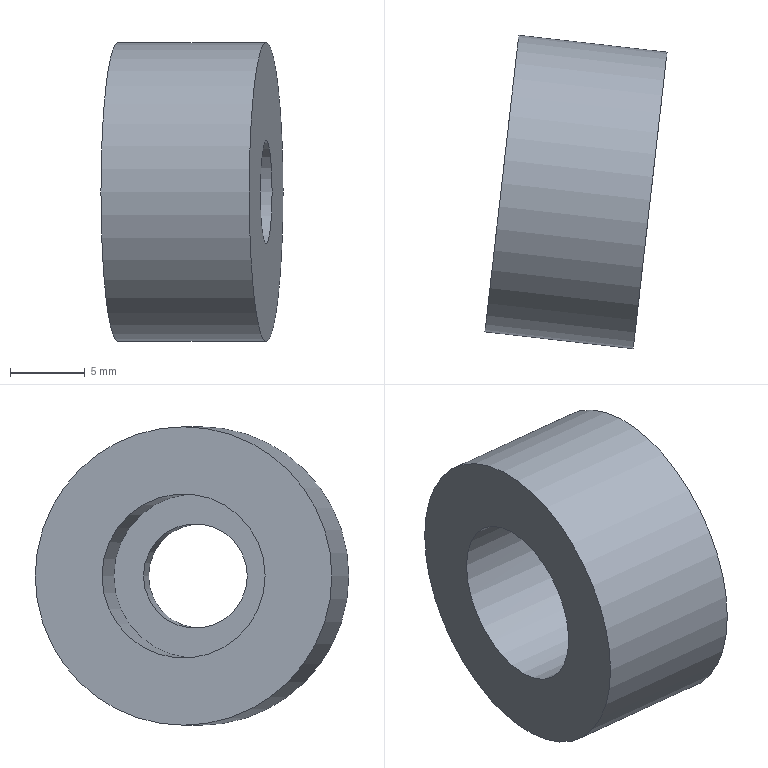Part | NX | features XQ 2 | 1 solid | 6 faces | box 12.2 x 21.003 x 20 mm | volume 2361 mm3 | plane 3 | cylinder 3 | commonest cylinder face diameters 7 x1 11 x1 20 x1
STEP:
#1=CARTESIAN_POINT('',(3212.648,-240.802,-118.5));
#2=VERTEX_POINT('',#1);
#3=CARTESIAN_POINT('',(3213.78,-230.866,-118.5));
#4=DIRECTION('',(-0.9936,0.1132,0.));
#5=DIRECTION('',(-0.1132,-0.9936,0.));
#6=AXIS2_PLACEMENT_3D('',#3,#4,#5);
#7=CIRCLE('',#6,10.);
#8=EDGE_CURVE('',#2,#2,#7,.T.);
#9=ORIENTED_EDGE('',*,*,#8,.T.);
#10=EDGE_LOOP('',(#9));
#11=FACE_BOUND('',#10,.T.);
#12=CARTESIAN_POINT('',(3213.85,-230.247,-123.965));
#13=VERTEX_POINT('',#12);
#14=CARTESIAN_POINT('',(3213.78,-230.866,-118.5));
#15=DIRECTION('',(0.9936,-0.1132,0.));
#16=DIRECTION('',(0.01281,0.1125,-0.9936));
#17=AXIS2_PLACEMENT_3D('',#14,#15,#16);
#18=CIRCLE('',#17,5.5);
#19=EDGE_CURVE('',#13,#13,#18,.T.);
#20=ORIENTED_EDGE('',*,*,#19,.T.);
#21=EDGE_LOOP('',(#20));
#22=FACE_BOUND('',#21,.T.);
#23=CARTESIAN_POINT('',(3213.78,-230.866,-118.5));
#24=DIRECTION('',(-0.9936,0.1132,0.));
#25=DIRECTION('',(0.1132,0.9936,0.));
#26=AXIS2_PLACEMENT_3D('',#23,#24,#25);
#27=PLANE('',#26);
#28=ADVANCED_FACE('',(#11,#22),#27,.T.);
#29=ORIENTED_EDGE('',*,*,#8,.F.);
#30=EDGE_LOOP('',(#29));
#31=FACE_BOUND('',#30,.T.);
#32=CARTESIAN_POINT('',(3222.584,-241.934,-118.5));
#33=VERTEX_POINT('',#32);
#34=CARTESIAN_POINT('',(3223.716,-231.998,-118.5));
#35=DIRECTION('',(-0.9936,0.1132,0.));
#36=DIRECTION('',(-0.1132,-0.9936,0.));
#37=AXIS2_PLACEMENT_3D('',#34,#35,#36);
#38=CIRCLE('',#37,10.);
#39=EDGE_CURVE('',#33,#33,#38,.T.);
#40=ORIENTED_EDGE('',*,*,#39,.T.);
#41=EDGE_LOOP('',(#40));
#42=FACE_BOUND('',#41,.T.);
#43=CARTESIAN_POINT('',(3213.78,-230.866,-118.5));
#44=DIRECTION('',(0.9936,-0.1132,0.));
#45=DIRECTION('',(-0.1132,-0.9936,0.));
#46=AXIS2_PLACEMENT_3D('',#43,#44,#45);
#47=CYLINDRICAL_SURFACE('',#46,10.);
#48=ADVANCED_FACE('',(#31,#42),#47,.T.);
#49=CARTESIAN_POINT('',(3223.319,-235.475,-118.5));
#50=VERTEX_POINT('',#49);
#51=CARTESIAN_POINT('',(3223.716,-231.998,-118.5));
#52=DIRECTION('',(-0.9936,0.1132,0.));
#53=DIRECTION('',(-0.1132,-0.9936,0.));
#54=AXIS2_PLACEMENT_3D('',#51,#52,#53);
#55=CIRCLE('',#54,3.5);
#56=EDGE_CURVE('',#50,#50,#55,.T.);
#57=ORIENTED_EDGE('',*,*,#56,.T.);
#58=EDGE_LOOP('',(#57));
#59=FACE_BOUND('',#58,.T.);
#60=ORIENTED_EDGE('',*,*,#39,.F.);
#61=EDGE_LOOP('',(#60));
#62=FACE_BOUND('',#61,.T.);
#63=CARTESIAN_POINT('',(3223.716,-231.998,-118.5));
#64=DIRECTION('',(-0.9936,0.1132,0.));
#65=DIRECTION('',(0.1132,0.9936,0.));
#66=AXIS2_PLACEMENT_3D('',#63,#64,#65);
#67=PLANE('',#66);
#68=ADVANCED_FACE('',(#59,#62),#67,.F.);
#69=CARTESIAN_POINT('',(3220.339,-235.136,-118.5));
#70=VERTEX_POINT('',#69);
#71=CARTESIAN_POINT('',(3220.735,-231.658,-118.5));
#72=DIRECTION('',(0.9936,-0.1132,0.));
#73=DIRECTION('',(-0.1132,-0.9936,0.));
#74=AXIS2_PLACEMENT_3D('',#71,#72,#73);
#75=CIRCLE('',#74,3.5);
#76=EDGE_CURVE('',#70,#70,#75,.T.);
#77=ORIENTED_EDGE('',*,*,#76,.F.);
#78=EDGE_LOOP('',(#77));
#79=FACE_BOUND('',#78,.T.);
#80=ORIENTED_EDGE('',*,*,#56,.F.);
#81=EDGE_LOOP('',(#80));
#82=FACE_BOUND('',#81,.T.);
#83=CARTESIAN_POINT('',(3213.78,-230.866,-118.5));
#84=DIRECTION('',(0.9936,-0.1132,0.));
#85=DIRECTION('',(-0.01281,-0.1125,0.9936));
#86=AXIS2_PLACEMENT_3D('',#83,#84,#85);
#87=CYLINDRICAL_SURFACE('',#86,3.5);
#88=ADVANCED_FACE('',(#79,#82),#87,.F.);
#89=ORIENTED_EDGE('',*,*,#76,.T.);
#90=EDGE_LOOP('',(#89));
#91=FACE_BOUND('',#90,.T.);
#92=CARTESIAN_POINT('',(3220.112,-237.123,-118.5));
#93=VERTEX_POINT('',#92);
#94=CARTESIAN_POINT('',(3220.735,-231.658,-118.5));
#95=DIRECTION('',(0.9936,-0.1132,0.));
#96=DIRECTION('',(-0.1132,-0.9936,0.));
#97=AXIS2_PLACEMENT_3D('',#94,#95,#96);
#98=CIRCLE('',#97,5.5);
#99=EDGE_CURVE('',#93,#93,#98,.T.);
#100=ORIENTED_EDGE('',*,*,#99,.F.);
#101=EDGE_LOOP('',(#100));
#102=FACE_BOUND('',#101,.T.);
#103=CARTESIAN_POINT('',(3212.924,-300.215,-81.5));
#104=DIRECTION('',(0.9936,-0.1132,0.));
#105=DIRECTION('',(-0.1132,-0.9936,0.));
#106=AXIS2_PLACEMENT_3D('',#103,#104,#105);
#107=PLANE('',#106);
#108=ADVANCED_FACE('',(#91,#102),#107,.F.);
#109=ORIENTED_EDGE('',*,*,#99,.T.);
#110=EDGE_LOOP('',(#109));
#111=FACE_BOUND('',#110,.T.);
#112=ORIENTED_EDGE('',*,*,#19,.F.);
#113=EDGE_LOOP('',(#112));
#114=FACE_BOUND('',#113,.T.);
#115=CARTESIAN_POINT('',(3213.78,-230.866,-118.5));
#116=DIRECTION('',(0.9936,-0.1132,0.));
#117=DIRECTION('',(-0.01281,-0.1125,0.9936));
#118=AXIS2_PLACEMENT_3D('',#115,#116,#117);
#119=CYLINDRICAL_SURFACE('',#118,5.5);
#120=ADVANCED_FACE('',(#111,#114),#119,.F.);
#121=CLOSED_SHELL('',(#28,#48,#68,#88,#108,#120));
#122=MANIFOLD_SOLID_BREP('',#121);
#123=(LENGTH_UNIT()NAMED_UNIT(*)SI_UNIT(.MILLI.,.METRE.));
#124=UNCERTAINTY_MEASURE_WITH_UNIT(LENGTH_MEASURE(0.00001),#123,'','');
#125=(NAMED_UNIT(*)PLANE_ANGLE_UNIT()SI_UNIT($,.RADIAN.));
#126=(NAMED_UNIT(*)SI_UNIT($,.STERADIAN.)SOLID_ANGLE_UNIT());
#127=(GEOMETRIC_REPRESENTATION_CONTEXT(3)GLOBAL_UNCERTAINTY_ASSIGNED_CONTEXT((#124))GLOBAL_UNIT_ASSIGNED_CONTEXT((#123,#125,#126))REPRESENTATION_CONTEXT('',''));
#128=ADVANCED_BREP_SHAPE_REPRESENTATION('',(#122),#127);